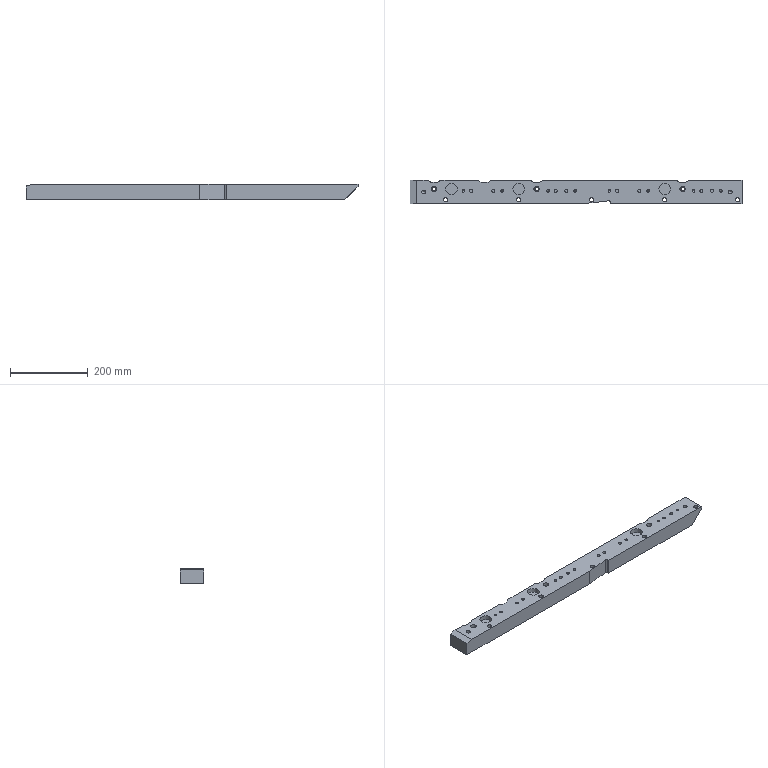Part | NX | features 22 2 | 1 solid | 97 faces | box 855 x 60 x 40 mm | volume 1889738 mm3 | cylinder 49 | plane 38 | cone 10 | commonest cylinder face diameters 14 x9 6.8 x8 8.001 x8 6 x6 11 x5 9 x3